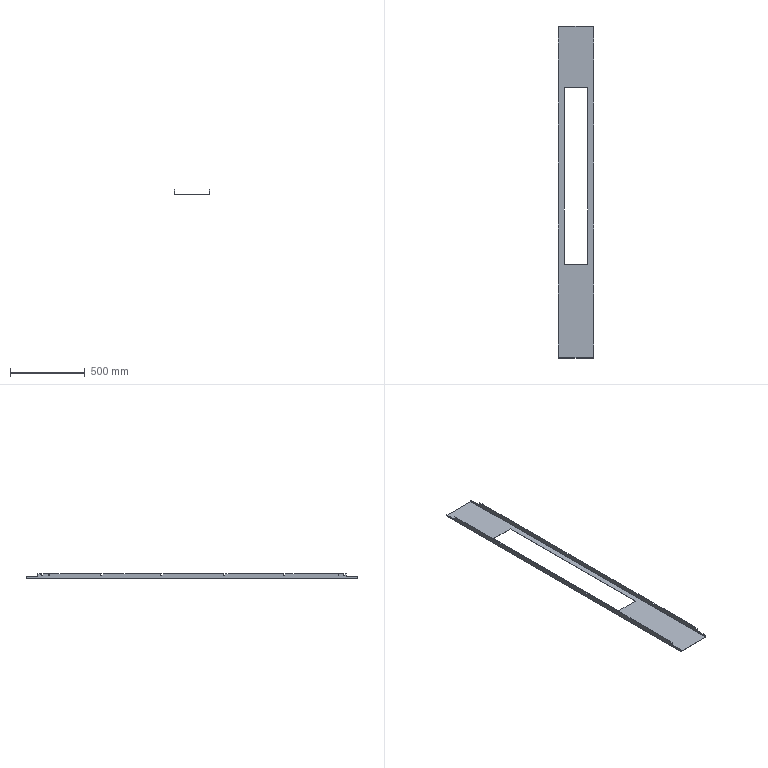Part | SolidWorks | features ICE 4, Chamfer 2, Cut 1, Fillet 1, FlatPattern 1, SMBaseFlange 1, SheetMetal 1 | 1 solid | 106 faces | box 235 x 2216 x 33 mm | volume 558098 mm3 | plane 70 | cylinder 36 | commonest cylinder face diameters 8.2 x24 6 x8 0.4 x2 2.8 x2